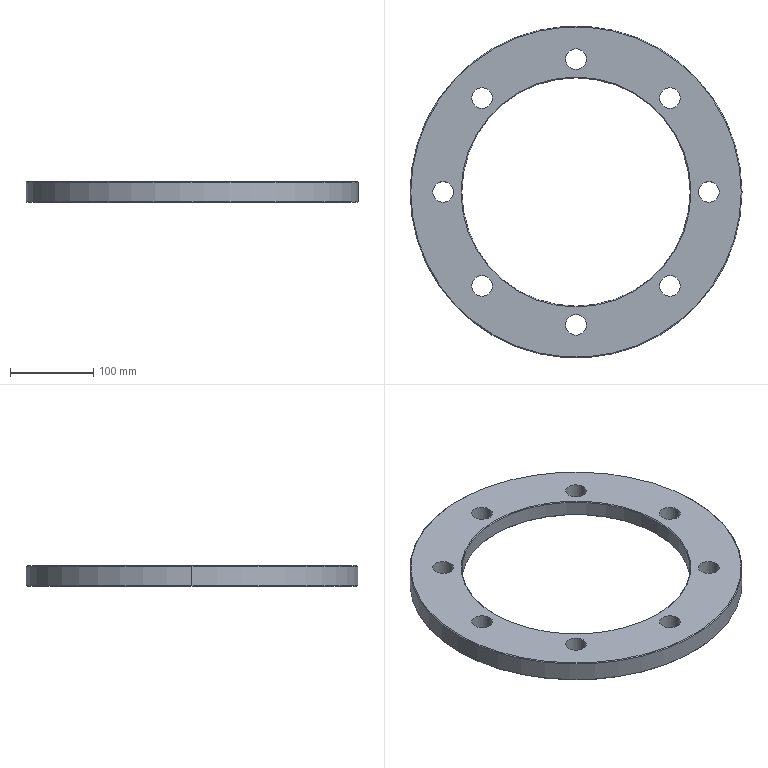Part | SolidWorks | features Chamfer 2, Extrusion 1, Fillet 1, ICE 1 | 1 solid | 37 faces | box 400 x 400 x 25 mm | volume 1378515 mm3 | cylinder 22 | cone 10 | plane 3 | torus 2 | commonest cylinder face diameters 25 x16 275 x2 355 x2 400 x2
STEP:
#1=CARTESIAN_POINT('',(177.5,0.,1.));
#2=VERTEX_POINT('',#1);
#3=CARTESIAN_POINT('',(-177.5,0.,1.));
#4=VERTEX_POINT('',#3);
#5=CARTESIAN_POINT('',(0.,0.,1.));
#6=DIRECTION('',(0.,0.,-1.));
#7=DIRECTION('',(1.,0.,0.));
#8=AXIS2_PLACEMENT_3D('',#5,#6,#7);
#9=CIRCLE('',#8,177.5);
#10=EDGE_CURVE('',#2,#4,#9,.T.);
#11=ORIENTED_EDGE('',*,*,#10,.F.);
#12=CARTESIAN_POINT('',(178.5,0.,0.));
#13=VERTEX_POINT('',#12);
#14=CARTESIAN_POINT('',(177.5,0.,1.));
#15=DIRECTION('',(0.7071,0.,-0.7071));
#16=VECTOR('',#15,1000.);
#17=LINE('',#14,#16);
#18=EDGE_CURVE('',#2,#13,#17,.T.);
#19=ORIENTED_EDGE('',*,*,#18,.T.);
#20=CARTESIAN_POINT('',(-178.5,0.,0.));
#21=VERTEX_POINT('',#20);
#22=CARTESIAN_POINT('',(0.,0.,0.));
#23=DIRECTION('',(0.,0.,1.));
#24=DIRECTION('',(1.,0.,0.));
#25=AXIS2_PLACEMENT_3D('',#22,#23,#24);
#26=CIRCLE('',#25,178.5);
#27=EDGE_CURVE('',#21,#13,#26,.T.);
#28=ORIENTED_EDGE('',*,*,#27,.F.);
#29=CARTESIAN_POINT('',(-177.5,0.,1.));
#30=DIRECTION('',(-0.7071,0.,-0.7071));
#31=VECTOR('',#30,1000.);
#32=LINE('',#29,#31);
#33=EDGE_CURVE('',#4,#21,#32,.T.);
#34=ORIENTED_EDGE('',*,*,#33,.F.);
#35=EDGE_LOOP('',(#11,#19,#28,#34));
#36=FACE_OUTER_BOUND('',#35,.T.);
#37=CARTESIAN_POINT('',(0.,0.,1.));
#38=DIRECTION('',(0.,0.,-1.));
#39=DIRECTION('',(-1.,0.,0.));
#40=AXIS2_PLACEMENT_3D('',#37,#38,#39);
#41=CONICAL_SURFACE('',#40,177.5,0.7854);
#42=ADVANCED_FACE('',(#36),#41,.F.);
#43=CARTESIAN_POINT('',(137.5,0.,6.));
#44=VERTEX_POINT('',#43);
#45=CARTESIAN_POINT('',(-137.5,0.,6.));
#46=VERTEX_POINT('',#45);
#47=CARTESIAN_POINT('',(0.,0.,6.));
#48=DIRECTION('',(0.,0.,-1.));
#49=DIRECTION('',(-1.,0.,0.));
#50=AXIS2_PLACEMENT_3D('',#47,#48,#49);
#51=CIRCLE('',#50,137.5);
#52=EDGE_CURVE('',#44,#46,#51,.T.);
#53=ORIENTED_EDGE('',*,*,#52,.F.);
#54=CARTESIAN_POINT('',(138.5,0.,5.));
#55=VERTEX_POINT('',#54);
#56=CARTESIAN_POINT('',(137.5,0.,6.));
#57=DIRECTION('',(0.7071,0.,-0.7071));
#58=VECTOR('',#57,1000.);
#59=LINE('',#56,#58);
#60=EDGE_CURVE('',#44,#55,#59,.T.);
#61=ORIENTED_EDGE('',*,*,#60,.T.);
#62=CARTESIAN_POINT('',(-138.5,0.,5.));
#63=VERTEX_POINT('',#62);
#64=CARTESIAN_POINT('',(0.,0.,5.));
#65=DIRECTION('',(0.,0.,1.));
#66=DIRECTION('',(-1.,0.,0.));
#67=AXIS2_PLACEMENT_3D('',#64,#65,#66);
#68=CIRCLE('',#67,138.5);
#69=EDGE_CURVE('',#63,#55,#68,.T.);
#70=ORIENTED_EDGE('',*,*,#69,.F.);
#71=CARTESIAN_POINT('',(-137.5,0.,6.));
#72=DIRECTION('',(-0.7071,0.,-0.7071));
#73=VECTOR('',#72,1000.);
#74=LINE('',#71,#73);
#75=EDGE_CURVE('',#46,#63,#74,.T.);
#76=ORIENTED_EDGE('',*,*,#75,.F.);
#77=EDGE_LOOP('',(#53,#61,#70,#76));
#78=FACE_OUTER_BOUND('',#77,.T.);
#79=CARTESIAN_POINT('',(0.,0.,6.));
#80=DIRECTION('',(0.,0.,-1.));
#81=DIRECTION('',(-1.,0.,0.));
#82=AXIS2_PLACEMENT_3D('',#79,#80,#81);
#83=CONICAL_SURFACE('',#82,137.5,0.7854);
#84=ADVANCED_FACE('',(#78),#83,.F.);
#85=CARTESIAN_POINT('',(175.5,0.,5.));
#86=VERTEX_POINT('',#85);
#87=CARTESIAN_POINT('',(-175.5,0.,5.));
#88=VERTEX_POINT('',#87);
#89=CARTESIAN_POINT('',(0.,0.,5.));
#90=DIRECTION('',(0.,0.,-1.));
#91=DIRECTION('',(-1.,0.,0.));
#92=AXIS2_PLACEMENT_3D('',#89,#90,#91);
#93=CIRCLE('',#92,175.5);
#94=EDGE_CURVE('',#86,#88,#93,.T.);
#95=ORIENTED_EDGE('',*,*,#94,.F.);
#96=CARTESIAN_POINT('',(177.5,0.,3.));
#97=VERTEX_POINT('',#96);
#98=CARTESIAN_POINT('',(175.5,0.,3.));
#99=DIRECTION('',(0.,1.,0.));
#100=DIRECTION('',(-1.,0.,0.));
#101=AXIS2_PLACEMENT_3D('',#98,#99,#100);
#102=CIRCLE('',#101,2.);
#103=EDGE_CURVE('',#86,#97,#102,.T.);
#104=ORIENTED_EDGE('',*,*,#103,.T.);
#105=CARTESIAN_POINT('',(-177.5,0.,3.));
#106=VERTEX_POINT('',#105);
#107=CARTESIAN_POINT('',(0.,0.,3.));
#108=DIRECTION('',(0.,0.,1.));
#109=DIRECTION('',(-1.,0.,0.));
#110=AXIS2_PLACEMENT_3D('',#107,#108,#109);
#111=CIRCLE('',#110,177.5);
#112=EDGE_CURVE('',#106,#97,#111,.T.);
#113=ORIENTED_EDGE('',*,*,#112,.F.);
#114=CARTESIAN_POINT('',(-175.5,0.,3.));
#115=DIRECTION('',(0.,-1.,0.));
#116=DIRECTION('',(1.,0.,0.));
#117=AXIS2_PLACEMENT_3D('',#114,#115,#116);
#118=CIRCLE('',#117,2.);
#119=EDGE_CURVE('',#88,#106,#118,.T.);
#120=ORIENTED_EDGE('',*,*,#119,.F.);
#121=EDGE_LOOP('',(#95,#104,#113,#120));
#122=FACE_OUTER_BOUND('',#121,.T.);
#123=CARTESIAN_POINT('',(0.,0.,3.));
#124=DIRECTION('',(0.,0.,-1.));
#125=DIRECTION('',(-1.,0.,0.));
#126=AXIS2_PLACEMENT_3D('',#123,#124,#125);
#127=TOROIDAL_SURFACE('',#126,175.5,2.);
#128=ADVANCED_FACE('',(#122),#127,.F.);
#129=ORIENTED_EDGE('',*,*,#112,.T.);
#130=CARTESIAN_POINT('',(177.5,0.,5.));
#131=DIRECTION('',(0.,0.,-1.));
#132=VECTOR('',#131,1000.);
#133=LINE('',#130,#132);
#134=EDGE_CURVE('',#97,#2,#133,.T.);
#135=ORIENTED_EDGE('',*,*,#134,.T.);
#136=ORIENTED_EDGE('',*,*,#10,.T.);
#137=CARTESIAN_POINT('',(-177.5,0.,5.));
#138=DIRECTION('',(0.,0.,-1.));
#139=VECTOR('',#138,1000.);
#140=LINE('',#137,#139);
#141=EDGE_CURVE('',#106,#4,#140,.T.);
#142=ORIENTED_EDGE('',*,*,#141,.F.);
#143=EDGE_LOOP('',(#129,#135,#136,#142));
#144=FACE_OUTER_BOUND('',#143,.T.);
#145=CARTESIAN_POINT('',(0.,0.,5.));
#146=DIRECTION('',(0.,0.,-1.));
#147=DIRECTION('',(-1.,0.,0.));
#148=AXIS2_PLACEMENT_3D('',#145,#146,#147);
#149=CYLINDRICAL_SURFACE('',#148,177.5);
#150=ADVANCED_FACE('',(#144),#149,.F.);
#151=CARTESIAN_POINT('',(199.,0.,25.));
#152=VERTEX_POINT('',#151);
#153=CARTESIAN_POINT('',(-199.,0.,25.));
#154=VERTEX_POINT('',#153);
#155=CARTESIAN_POINT('',(0.,0.,25.));
#156=DIRECTION('',(0.,0.,1.));
#157=DIRECTION('',(1.,0.,0.));
#158=AXIS2_PLACEMENT_3D('',#155,#156,#157);
#159=CIRCLE('',#158,199.);
#160=EDGE_CURVE('',#152,#154,#159,.T.);
#161=ORIENTED_EDGE('',*,*,#160,.F.);
#162=CARTESIAN_POINT('',(200.,0.,24.));
#163=VERTEX_POINT('',#162);
#164=CARTESIAN_POINT('',(199.,0.,25.));
#165=DIRECTION('',(0.7071,0.,-0.7071));
#166=VECTOR('',#165,1000.);
#167=LINE('',#164,#166);
#168=EDGE_CURVE('',#152,#163,#167,.T.);
#169=ORIENTED_EDGE('',*,*,#168,.T.);
#170=CARTESIAN_POINT('',(-200.,0.,24.));
#171=VERTEX_POINT('',#170);
#172=CARTESIAN_POINT('',(0.,0.,24.));
#173=DIRECTION('',(0.,0.,-1.));
#174=DIRECTION('',(1.,0.,0.));
#175=AXIS2_PLACEMENT_3D('',#172,#173,#174);
#176=CIRCLE('',#175,200.);
#177=EDGE_CURVE('',#171,#163,#176,.T.);
#178=ORIENTED_EDGE('',*,*,#177,.F.);
#179=CARTESIAN_POINT('',(-199.,0.,25.));
#180=DIRECTION('',(-0.7071,0.,-0.7071));
#181=VECTOR('',#180,1000.);
#182=LINE('',#179,#181);
#183=EDGE_CURVE('',#154,#171,#182,.T.);
#184=ORIENTED_EDGE('',*,*,#183,.F.);
#185=EDGE_LOOP('',(#161,#169,#178,#184));
#186=FACE_OUTER_BOUND('',#185,.T.);
#187=CARTESIAN_POINT('',(0.,0.,25.));
#188=DIRECTION('',(0.,0.,-1.));
#189=DIRECTION('',(-1.,0.,0.));
#190=AXIS2_PLACEMENT_3D('',#187,#188,#189);
#191=CONICAL_SURFACE('',#190,199.,0.7854);
#192=ADVANCED_FACE('',(#186),#191,.T.);
#193=CARTESIAN_POINT('',(-199.,0.,0.));
#194=VERTEX_POINT('',#193);
#195=CARTESIAN_POINT('',(199.,0.,0.));
#196=VERTEX_POINT('',#195);
#197=CARTESIAN_POINT('',(0.,0.,0.));
#198=DIRECTION('',(0.,0.,-1.));
#199=DIRECTION('',(1.,0.,0.));
#200=AXIS2_PLACEMENT_3D('',#197,#198,#199);
#201=CIRCLE('',#200,199.);
#202=EDGE_CURVE('',#194,#196,#201,.T.);
#203=ORIENTED_EDGE('',*,*,#202,.F.);
#204=CARTESIAN_POINT('',(-200.,0.,1.));
#205=VERTEX_POINT('',#204);
#206=CARTESIAN_POINT('',(-200.,0.,1.));
#207=DIRECTION('',(-0.7071,0.,0.7071));
#208=VECTOR('',#207,1000.);
#209=LINE('',#206,#208);
#210=EDGE_CURVE('',#194,#205,#209,.T.);
#211=ORIENTED_EDGE('',*,*,#210,.T.);
#212=CARTESIAN_POINT('',(200.,0.,1.));
#213=VERTEX_POINT('',#212);
#214=CARTESIAN_POINT('',(0.,0.,1.));
#215=DIRECTION('',(0.,0.,1.));
#216=DIRECTION('',(1.,0.,0.));
#217=AXIS2_PLACEMENT_3D('',#214,#215,#216);
#218=CIRCLE('',#217,200.);
#219=EDGE_CURVE('',#213,#205,#218,.T.);
#220=ORIENTED_EDGE('',*,*,#219,.F.);
#221=CARTESIAN_POINT('',(200.,0.,1.));
#222=DIRECTION('',(0.7071,0.,0.7071));
#223=VECTOR('',#222,1000.);
#224=LINE('',#221,#223);
#225=EDGE_CURVE('',#196,#213,#224,.T.);
#226=ORIENTED_EDGE('',*,*,#225,.F.);
#227=EDGE_LOOP('',(#203,#211,#220,#226));
#228=FACE_OUTER_BOUND('',#227,.T.);
#229=CARTESIAN_POINT('',(0.,0.,1.));
#230=DIRECTION('',(0.,0.,1.));
#231=DIRECTION('',(1.,0.,0.));
#232=AXIS2_PLACEMENT_3D('',#229,#230,#231);
#233=CONICAL_SURFACE('',#232,200.,0.7854);
#234=ADVANCED_FACE('',(#228),#233,.T.);
#235=CARTESIAN_POINT('',(-137.5,0.,24.));
#236=VERTEX_POINT('',#235);
#237=CARTESIAN_POINT('',(137.5,0.,24.));
#238=VERTEX_POINT('',#237);
#239=CARTESIAN_POINT('',(0.,0.,24.));
#240=DIRECTION('',(0.,0.,1.));
#241=DIRECTION('',(1.,0.,0.));
#242=AXIS2_PLACEMENT_3D('',#239,#240,#241);
#243=CIRCLE('',#242,137.5);
#244=EDGE_CURVE('',#236,#238,#243,.T.);
#245=ORIENTED_EDGE('',*,*,#244,.F.);
#246=CARTESIAN_POINT('',(-138.5,0.,25.));
#247=VERTEX_POINT('',#246);
#248=CARTESIAN_POINT('',(-137.5,0.,24.));
#249=DIRECTION('',(-0.7071,0.,0.7071));
#250=VECTOR('',#249,1000.);
#251=LINE('',#248,#250);
#252=EDGE_CURVE('',#236,#247,#251,.T.);
#253=ORIENTED_EDGE('',*,*,#252,.T.);
#254=CARTESIAN_POINT('',(138.5,0.,25.));
#255=VERTEX_POINT('',#254);
#256=CARTESIAN_POINT('',(0.,0.,25.));
#257=DIRECTION('',(0.,0.,-1.));
#258=DIRECTION('',(1.,0.,0.));
#259=AXIS2_PLACEMENT_3D('',#256,#257,#258);
#260=CIRCLE('',#259,138.5);
#261=EDGE_CURVE('',#255,#247,#260,.T.);
#262=ORIENTED_EDGE('',*,*,#261,.F.);
#263=CARTESIAN_POINT('',(137.5,0.,24.));
#264=DIRECTION('',(0.7071,0.,0.7071));
#265=VECTOR('',#264,1000.);
#266=LINE('',#263,#265);
#267=EDGE_CURVE('',#238,#255,#266,.T.);
#268=ORIENTED_EDGE('',*,*,#267,.F.);
#269=EDGE_LOOP('',(#245,#253,#262,#268));
#270=FACE_OUTER_BOUND('',#269,.T.);
#271=CARTESIAN_POINT('',(0.,0.,24.));
#272=DIRECTION('',(0.,0.,1.));
#273=DIRECTION('',(1.,0.,0.));
#274=AXIS2_PLACEMENT_3D('',#271,#272,#273);
#275=CONICAL_SURFACE('',#274,137.5,0.7854);
#276=ADVANCED_FACE('',(#270),#275,.F.);
#277=ORIENTED_EDGE('',*,*,#177,.T.);
#278=CARTESIAN_POINT('',(200.,0.,25.));
#279=DIRECTION('',(0.,0.,-1.));
#280=VECTOR('',#279,1000.);
#281=LINE('',#278,#280);
#282=EDGE_CURVE('',#163,#213,#281,.T.);
#283=ORIENTED_EDGE('',*,*,#282,.T.);
#284=ORIENTED_EDGE('',*,*,#219,.T.);
#285=CARTESIAN_POINT('',(-200.,0.,25.));
#286=DIRECTION('',(0.,0.,-1.));
#287=VECTOR('',#286,1000.);
#288=LINE('',#285,#287);
#289=EDGE_CURVE('',#171,#205,#288,.T.);
#290=ORIENTED_EDGE('',*,*,#289,.F.);
#291=EDGE_LOOP('',(#277,#283,#284,#290));
#292=FACE_OUTER_BOUND('',#291,.T.);
#293=CARTESIAN_POINT('',(0.,0.,25.));
#294=DIRECTION('',(0.,0.,-1.));
#295=DIRECTION('',(-1.,0.,0.));
#296=AXIS2_PLACEMENT_3D('',#293,#294,#295);
#297=CYLINDRICAL_SURFACE('',#296,200.);
#298=ADVANCED_FACE('',(#292),#297,.T.);
#299=CARTESIAN_POINT('',(-125.637,113.137,25.));
#300=VERTEX_POINT('',#299);
#301=CARTESIAN_POINT('',(-100.637,113.137,25.));
#302=VERTEX_POINT('',#301);
#303=CARTESIAN_POINT('',(-113.137,113.137,25.));
#304=DIRECTION('',(0.,0.,1.));
#305=DIRECTION('',(1.,0.,0.));
#306=AXIS2_PLACEMENT_3D('',#303,#304,#305);
#307=CIRCLE('',#306,12.5);
#308=EDGE_CURVE('',#300,#302,#307,.T.);
#309=ORIENTED_EDGE('',*,*,#308,.T.);
#310=CARTESIAN_POINT('',(-100.637,113.137,5.));
#311=VERTEX_POINT('',#310);
#312=CARTESIAN_POINT('',(-100.637,113.137,25.));
#313=DIRECTION('',(0.,0.,-1.));
#314=VECTOR('',#313,1000.);
#315=LINE('',#312,#314);
#316=EDGE_CURVE('',#302,#311,#315,.T.);
#317=ORIENTED_EDGE('',*,*,#316,.T.);
#318=CARTESIAN_POINT('',(-125.637,113.137,5.));
#319=VERTEX_POINT('',#318);
#320=CARTESIAN_POINT('',(-113.137,113.137,5.));
#321=DIRECTION('',(0.,0.,-1.));
#322=DIRECTION('',(-1.,0.,0.));
#323=AXIS2_PLACEMENT_3D('',#320,#321,#322);
#324=CIRCLE('',#323,12.5);
#325=EDGE_CURVE('',#311,#319,#324,.T.);
#326=ORIENTED_EDGE('',*,*,#325,.T.);
#327=CARTESIAN_POINT('',(-125.637,113.137,25.));
#328=DIRECTION('',(0.,0.,-1.));
#329=VECTOR('',#328,1000.);
#330=LINE('',#327,#329);
#331=EDGE_CURVE('',#300,#319,#330,.T.);
#332=ORIENTED_EDGE('',*,*,#331,.F.);
#333=EDGE_LOOP('',(#309,#317,#326,#332));
#334=FACE_OUTER_BOUND('',#333,.T.);
#335=CARTESIAN_POINT('',(-113.137,113.137,25.));
#336=DIRECTION('',(0.,0.,-1.));
#337=DIRECTION('',(-1.,0.,0.));
#338=AXIS2_PLACEMENT_3D('',#335,#336,#337);
#339=CYLINDRICAL_SURFACE('',#338,12.5);
#340=ADVANCED_FACE('',(#334),#339,.F.);
#341=CARTESIAN_POINT('',(-172.5,0.,25.));
#342=VERTEX_POINT('',#341);
#343=CARTESIAN_POINT('',(-147.5,0.,25.));
#344=VERTEX_POINT('',#343);
#345=CARTESIAN_POINT('',(-160.,0.,25.));
#346=DIRECTION('',(0.,0.,1.));
#347=DIRECTION('',(1.,0.,0.));
#348=AXIS2_PLACEMENT_3D('',#345,#346,#347);
#349=CIRCLE('',#348,12.5);
#350=EDGE_CURVE('',#342,#344,#349,.T.);
#351=ORIENTED_EDGE('',*,*,#350,.T.);
#352=CARTESIAN_POINT('',(-147.5,0.,5.));
#353=VERTEX_POINT('',#352);
#354=CARTESIAN_POINT('',(-147.5,0.,25.));
#355=DIRECTION('',(0.,0.,-1.));
#356=VECTOR('',#355,1000.);
#357=LINE('',#354,#356);
#358=EDGE_CURVE('',#344,#353,#357,.T.);
#359=ORIENTED_EDGE('',*,*,#358,.T.);
#360=CARTESIAN_POINT('',(-172.5,0.,5.));
#361=VERTEX_POINT('',#360);
#362=CARTESIAN_POINT('',(-160.,0.,5.));
#363=DIRECTION('',(0.,0.,-1.));
#364=DIRECTION('',(-1.,0.,0.));
#365=AXIS2_PLACEMENT_3D('',#362,#363,#364);
#366=CIRCLE('',#365,12.5);
#367=EDGE_CURVE('',#353,#361,#366,.T.);
#368=ORIENTED_EDGE('',*,*,#367,.T.);
#369=CARTESIAN_POINT('',(-172.5,0.,25.));
#370=DIRECTION('',(0.,0.,-1.));
#371=VECTOR('',#370,1000.);
#372=LINE('',#369,#371);
#373=EDGE_CURVE('',#342,#361,#372,.T.);
#374=ORIENTED_EDGE('',*,*,#373,.F.);
#375=EDGE_LOOP('',(#351,#359,#368,#374));
#376=FACE_OUTER_BOUND('',#375,.T.);
#377=CARTESIAN_POINT('',(-160.,0.,25.));
#378=DIRECTION('',(0.,0.,-1.));
#379=DIRECTION('',(-1.,0.,0.));
#380=AXIS2_PLACEMENT_3D('',#377,#378,#379);
#381=CYLINDRICAL_SURFACE('',#380,12.5);
#382=ADVANCED_FACE('',(#376),#381,.F.);
#383=CARTESIAN_POINT('',(-125.637,-113.137,25.));
#384=VERTEX_POINT('',#383);
#385=CARTESIAN_POINT('',(-100.637,-113.137,25.));
#386=VERTEX_POINT('',#385);
#387=CARTESIAN_POINT('',(-113.137,-113.137,25.));
#388=DIRECTION('',(0.,0.,1.));
#389=DIRECTION('',(1.,0.,0.));
#390=AXIS2_PLACEMENT_3D('',#387,#388,#389);
#391=CIRCLE('',#390,12.5);
#392=EDGE_CURVE('',#384,#386,#391,.T.);
#393=ORIENTED_EDGE('',*,*,#392,.T.);
#394=CARTESIAN_POINT('',(-100.637,-113.137,5.));
#395=VERTEX_POINT('',#394);
#396=CARTESIAN_POINT('',(-100.637,-113.137,25.));
#397=DIRECTION('',(0.,0.,-1.));
#398=VECTOR('',#397,1000.);
#399=LINE('',#396,#398);
#400=EDGE_CURVE('',#386,#395,#399,.T.);
#401=ORIENTED_EDGE('',*,*,#400,.T.);
#402=CARTESIAN_POINT('',(-125.637,-113.137,5.));
#403=VERTEX_POINT('',#402);
#404=CARTESIAN_POINT('',(-113.137,-113.137,5.));
#405=DIRECTION('',(0.,0.,-1.));
#406=DIRECTION('',(-1.,0.,0.));
#407=AXIS2_PLACEMENT_3D('',#404,#405,#406);
#408=CIRCLE('',#407,12.5);
#409=EDGE_CURVE('',#395,#403,#408,.T.);
#410=ORIENTED_EDGE('',*,*,#409,.T.);
#411=CARTESIAN_POINT('',(-125.637,-113.137,25.));
#412=DIRECTION('',(0.,0.,-1.));
#413=VECTOR('',#412,1000.);
#414=LINE('',#411,#413);
#415=EDGE_CURVE('',#384,#403,#414,.T.);
#416=ORIENTED_EDGE('',*,*,#415,.F.);
#417=EDGE_LOOP('',(#393,#401,#410,#416));
#418=FACE_OUTER_BOUND('',#417,.T.);
#419=CARTESIAN_POINT('',(-113.137,-113.137,25.));
#420=DIRECTION('',(0.,0.,-1.));
#421=DIRECTION('',(-1.,0.,0.));
#422=AXIS2_PLACEMENT_3D('',#419,#420,#421);
#423=CYLINDRICAL_SURFACE('',#422,12.5);
#424=ADVANCED_FACE('',(#418),#423,.F.);
#425=CARTESIAN_POINT('',(-12.5,-160.,25.));
#426=VERTEX_POINT('',#425);
#427=CARTESIAN_POINT('',(12.5,-160.,25.));
#428=VERTEX_POINT('',#427);
#429=CARTESIAN_POINT('',(0.,-160.,25.));
#430=DIRECTION('',(0.,0.,1.));
#431=DIRECTION('',(1.,0.,0.));
#432=AXIS2_PLACEMENT_3D('',#429,#430,#431);
#433=CIRCLE('',#432,12.5);
#434=EDGE_CURVE('',#426,#428,#433,.T.);
#435=ORIENTED_EDGE('',*,*,#434,.T.);
#436=CARTESIAN_POINT('',(12.5,-160.,5.));
#437=VERTEX_POINT('',#436);
#438=CARTESIAN_POINT('',(12.5,-160.,25.));
#439=DIRECTION('',(0.,0.,-1.));
#440=VECTOR('',#439,1000.);
#441=LINE('',#438,#440);
#442=EDGE_CURVE('',#428,#437,#441,.T.);
#443=ORIENTED_EDGE('',*,*,#442,.T.);
#444=CARTESIAN_POINT('',(-12.5,-160.,5.));
#445=VERTEX_POINT('',#444);
#446=CARTESIAN_POINT('',(0.,-160.,5.));
#447=DIRECTION('',(0.,0.,-1.));
#448=DIRECTION('',(-1.,0.,0.));
#449=AXIS2_PLACEMENT_3D('',#446,#447,#448);
#450=CIRCLE('',#449,12.5);
#451=EDGE_CURVE('',#437,#445,#450,.T.);
#452=ORIENTED_EDGE('',*,*,#451,.T.);
#453=CARTESIAN_POINT('',(-12.5,-160.,25.));
#454=DIRECTION('',(0.,0.,-1.));
#455=VECTOR('',#454,1000.);
#456=LINE('',#453,#455);
#457=EDGE_CURVE('',#426,#445,#456,.T.);
#458=ORIENTED_EDGE('',*,*,#457,.F.);
#459=EDGE_LOOP('',(#435,#443,#452,#458));
#460=FACE_OUTER_BOUND('',#459,.T.);
#461=CARTESIAN_POINT('',(0.,-160.,25.));
#462=DIRECTION('',(0.,0.,-1.));
#463=DIRECTION('',(-1.,0.,0.));
#464=AXIS2_PLACEMENT_3D('',#461,#462,#463);
#465=CYLINDRICAL_SURFACE('',#464,12.5);
#466=ADVANCED_FACE('',(#460),#465,.F.);
#467=CARTESIAN_POINT('',(100.637,-113.137,25.));
#468=VERTEX_POINT('',#467);
#469=CARTESIAN_POINT('',(125.637,-113.137,25.));
#470=VERTEX_POINT('',#469);
#471=CARTESIAN_POINT('',(113.137,-113.137,25.));
#472=DIRECTION('',(0.,0.,1.));
#473=DIRECTION('',(1.,0.,0.));
#474=AXIS2_PLACEMENT_3D('',#471,#472,#473);
#475=CIRCLE('',#474,12.5);
#476=EDGE_CURVE('',#468,#470,#475,.T.);
#477=ORIENTED_EDGE('',*,*,#476,.T.);
#478=CARTESIAN_POINT('',(125.637,-113.137,5.));
#479=VERTEX_POINT('',#478);
#480=CARTESIAN_POINT('',(125.637,-113.137,25.));
#481=DIRECTION('',(0.,0.,-1.));
#482=VECTOR('',#481,1000.);
#483=LINE('',#480,#482);
#484=EDGE_CURVE('',#470,#479,#483,.T.);
#485=ORIENTED_EDGE('',*,*,#484,.T.);
#486=CARTESIAN_POINT('',(100.637,-113.137,5.));
#487=VERTEX_POINT('',#486);
#488=CARTESIAN_POINT('',(113.137,-113.137,5.));
#489=DIRECTION('',(0.,0.,-1.));
#490=DIRECTION('',(-1.,0.,0.));
#491=AXIS2_PLACEMENT_3D('',#488,#489,#490);
#492=CIRCLE('',#491,12.5);
#493=EDGE_CURVE('',#479,#487,#492,.T.);
#494=ORIENTED_EDGE('',*,*,#493,.T.);
#495=CARTESIAN_POINT('',(100.637,-113.137,25.));
#496=DIRECTION('',(0.,0.,-1.));
#497=VECTOR('',#496,1000.);
#498=LINE('',#495,#497);
#499=EDGE_CURVE('',#468,#487,#498,.T.);
#500=ORIENTED_EDGE('',*,*,#499,.F.);
#501=EDGE_LOOP('',(#477,#485,#494,#500));
#502=FACE_OUTER_BOUND('',#501,.T.);
#503=CARTESIAN_POINT('',(113.137,-113.137,25.));
#504=DIRECTION('',(0.,0.,-1.));
#505=DIRECTION('',(-1.,0.,0.));
#506=AXIS2_PLACEMENT_3D('',#503,#504,#505);
#507=CYLINDRICAL_SURFACE('',#506,12.5);
#508=ADVANCED_FACE('',(#502),#507,.F.);
#509=CARTESIAN_POINT('',(147.5,0.,25.));
#510=VERTEX_POINT('',#509);
#511=CARTESIAN_POINT('',(172.5,0.,25.));
#512=VERTEX_POINT('',#511);
#513=CARTESIAN_POINT('',(160.,0.,25.));
#514=DIRECTION('',(0.,0.,1.));
#515=DIRECTION('',(1.,0.,0.));
#516=AXIS2_PLACEMENT_3D('',#513,#514,#515);
#517=CIRCLE('',#516,12.5);
#518=EDGE_CURVE('',#510,#512,#517,.T.);
#519=ORIENTED_EDGE('',*,*,#518,.T.);
#520=CARTESIAN_POINT('',(172.5,0.,5.));
#521=VERTEX_POINT('',#520);
#522=CARTESIAN_POINT('',(172.5,0.,25.));
#523=DIRECTION('',(0.,0.,-1.));
#524=VECTOR('',#523,1000.);
#525=LINE('',#522,#524);
#526=EDGE_CURVE('',#512,#521,#525,.T.);
#527=ORIENTED_EDGE('',*,*,#526,.T.);
#528=CARTESIAN_POINT('',(147.5,0.,5.));
#529=VERTEX_POINT('',#528);
#530=CARTESIAN_POINT('',(160.,0.,5.));
#531=DIRECTION('',(0.,0.,-1.));
#532=DIRECTION('',(-1.,0.,0.));
#533=AXIS2_PLACEMENT_3D('',#530,#531,#532);
#534=CIRCLE('',#533,12.5);
#535=EDGE_CURVE('',#521,#529,#534,.T.);
#536=ORIENTED_EDGE('',*,*,#535,.T.);
#537=CARTESIAN_POINT('',(147.5,0.,25.));
#538=DIRECTION('',(0.,0.,-1.));
#539=VECTOR('',#538,1000.);
#540=LINE('',#537,#539);
#541=EDGE_CURVE('',#510,#529,#540,.T.);
#542=ORIENTED_EDGE('',*,*,#541,.F.);
#543=EDGE_LOOP('',(#519,#527,#536,#542));
#544=FACE_OUTER_BOUND('',#543,.T.);
#545=CARTESIAN_POINT('',(160.,0.,25.));
#546=DIRECTION('',(0.,0.,-1.));
#547=DIRECTION('',(-1.,0.,0.));
#548=AXIS2_PLACEMENT_3D('',#545,#546,#547);
#549=CYLINDRICAL_SURFACE('',#548,12.5);
#550=ADVANCED_FACE('',(#544),#549,.F.);
#551=CARTESIAN_POINT('',(100.637,113.137,25.));
#552=VERTEX_POINT('',#551);
#553=CARTESIAN_POINT('',(125.637,113.137,25.));
#554=VERTEX_POINT('',#553);
#555=CARTESIAN_POINT('',(113.137,113.137,25.));
#556=DIRECTION('',(0.,0.,1.));
#557=DIRECTION('',(1.,0.,0.));
#558=AXIS2_PLACEMENT_3D('',#555,#556,#557);
#559=CIRCLE('',#558,12.5);
#560=EDGE_CURVE('',#552,#554,#559,.T.);
#561=ORIENTED_EDGE('',*,*,#560,.T.);
#562=CARTESIAN_POINT('',(125.637,113.137,5.));
#563=VERTEX_POINT('',#562);
#564=CARTESIAN_POINT('',(125.637,113.137,25.));
#565=DIRECTION('',(0.,0.,-1.));
#566=VECTOR('',#565,1000.);
#567=LINE('',#564,#566);
#568=EDGE_CURVE('',#554,#563,#567,.T.);
#569=ORIENTED_EDGE('',*,*,#568,.T.);
#570=CARTESIAN_POINT('',(100.637,113.137,5.));
#571=VERTEX_POINT('',#570);
#572=CARTESIAN_POINT('',(113.137,113.137,5.));
#573=DIRECTION('',(0.,0.,-1.));
#574=DIRECTION('',(-1.,0.,0.));
#575=AXIS2_PLACEMENT_3D('',#572,#573,#574);
#576=CIRCLE('',#575,12.5);
#577=EDGE_CURVE('',#563,#571,#576,.T.);
#578=ORIENTED_EDGE('',*,*,#577,.T.);
#579=CARTESIAN_POINT('',(100.637,113.137,25.));
#580=DIRECTION('',(0.,0.,-1.));
#581=VECTOR('',#580,1000.);
#582=LINE('',#579,#581);
#583=EDGE_CURVE('',#552,#571,#582,.T.);
#584=ORIENTED_EDGE('',*,*,#583,.F.);
#585=EDGE_LOOP('',(#561,#569,#578,#584));
#586=FACE_OUTER_BOUND('',#585,.T.);
#587=CARTESIAN_POINT('',(113.137,113.137,25.));
#588=DIRECTION('',(0.,0.,-1.));
#589=DIRECTION('',(-1.,0.,0.));
#590=AXIS2_PLACEMENT_3D('',#587,#588,#589);
#591=CYLINDRICAL_SURFACE('',#590,12.5);
#592=ADVANCED_FACE('',(#586),#591,.F.);
#593=CARTESIAN_POINT('',(-12.5,160.,25.));
#594=VERTEX_POINT('',#593);
#595=CARTESIAN_POINT('',(12.5,160.,25.));
#596=VERTEX_POINT('',#595);
#597=CARTESIAN_POINT('',(0.,160.,25.));
#598=DIRECTION('',(0.,0.,1.));
#599=DIRECTION('',(1.,0.,0.));
#600=AXIS2_PLACEMENT_3D('',#597,#598,#599);
#601=CIRCLE('',#600,12.5);
#602=EDGE_CURVE('',#594,#596,#601,.T.);
#603=ORIENTED_EDGE('',*,*,#602,.T.);
#604=CARTESIAN_POINT('',(12.5,160.,5.));
#605=VERTEX_POINT('',#604);
#606=CARTESIAN_POINT('',(12.5,160.,25.));
#607=DIRECTION('',(0.,0.,-1.));
#608=VECTOR('',#607,1000.);
#609=LINE('',#606,#608);
#610=EDGE_CURVE('',#596,#605,#609,.T.);
#611=ORIENTED_EDGE('',*,*,#610,.T.);
#612=CARTESIAN_POINT('',(-12.5,160.,5.));
#613=VERTEX_POINT('',#612);
#614=CARTESIAN_POINT('',(0.,160.,5.));
#615=DIRECTION('',(0.,0.,-1.));
#616=DIRECTION('',(-1.,0.,0.));
#617=AXIS2_PLACEMENT_3D('',#614,#615,#616);
#618=CIRCLE('',#617,12.5);
#619=EDGE_CURVE('',#605,#613,#618,.T.);
#620=ORIENTED_EDGE('',*,*,#619,.T.);
#621=CARTESIAN_POINT('',(-12.5,160.,25.));
#622=DIRECTION('',(0.,0.,-1.));
#623=VECTOR('',#622,1000.);
#624=LINE('',#621,#623);
#625=EDGE_CURVE('',#594,#613,#624,.T.);
#626=ORIENTED_EDGE('',*,*,#625,.F.);
#627=EDGE_LOOP('',(#603,#611,#620,#626));
#628=FACE_OUTER_BOUND('',#627,.T.);
#629=CARTESIAN_POINT('',(0.,160.,25.));
#630=DIRECTION('',(0.,0.,-1.));
#631=DIRECTION('',(-1.,0.,0.));
#632=AXIS2_PLACEMENT_3D('',#629,#630,#631);
#633=CYLINDRICAL_SURFACE('',#632,12.5);
#634=ADVANCED_FACE('',(#628),#633,.F.);
#635=ORIENTED_EDGE('',*,*,#244,.T.);
#636=CARTESIAN_POINT('',(137.5,0.,25.));
#637=DIRECTION('',(0.,0.,-1.));
#638=VECTOR('',#637,1000.);
#639=LINE('',#636,#638);
#640=EDGE_CURVE('',#238,#44,#639,.T.);
#641=ORIENTED_EDGE('',*,*,#640,.T.);
#642=ORIENTED_EDGE('',*,*,#52,.T.);
#643=CARTESIAN_POINT('',(-137.5,0.,25.));
#644=DIRECTION('',(0.,0.,-1.));
#645=VECTOR('',#644,1000.);
#646=LINE('',#643,#645);
#647=EDGE_CURVE('',#236,#46,#646,.T.);
#648=ORIENTED_EDGE('',*,*,#647,.F.);
#649=EDGE_LOOP('',(#635,#641,#642,#648));
#650=FACE_OUTER_BOUND('',#649,.T.);
#651=CARTESIAN_POINT('',(0.,0.,25.));
#652=DIRECTION('',(0.,0.,-1.));
#653=DIRECTION('',(-1.,0.,0.));
#654=AXIS2_PLACEMENT_3D('',#651,#652,#653);
#655=CYLINDRICAL_SURFACE('',#654,137.5);
#656=ADVANCED_FACE('',(#650),#655,.F.);
#657=ORIENTED_EDGE('',*,*,#640,.F.);
#658=CARTESIAN_POINT('',(0.,0.,24.));
#659=DIRECTION('',(0.,0.,1.));
#660=DIRECTION('',(1.,0.,0.));
#661=AXIS2_PLACEMENT_3D('',#658,#659,#660);
#662=CIRCLE('',#661,137.5);
#663=EDGE_CURVE('',#238,#236,#662,.T.);
#664=ORIENTED_EDGE('',*,*,#663,.T.);
#665=ORIENTED_EDGE('',*,*,#647,.T.);
#666=CARTESIAN_POINT('',(0.,0.,6.));
#667=DIRECTION('',(0.,0.,-1.));
#668=DIRECTION('',(-1.,0.,0.));
#669=AXIS2_PLACEMENT_3D('',#666,#667,#668);
#670=CIRCLE('',#669,137.5);
#671=EDGE_CURVE('',#46,#44,#670,.T.);
#672=ORIENTED_EDGE('',*,*,#671,.T.);
#673=EDGE_LOOP('',(#657,#664,#665,#672));
#674=FACE_OUTER_BOUND('',#673,.T.);
#675=CARTESIAN_POINT('',(0.,0.,25.));
#676=DIRECTION('',(0.,0.,-1.));
#677=DIRECTION('',(-1.,0.,0.));
#678=AXIS2_PLACEMENT_3D('',#675,#676,#677);
#679=CYLINDRICAL_SURFACE('',#678,137.5);
#680=ADVANCED_FACE('',(#674),#679,.F.);
#681=ORIENTED_EDGE('',*,*,#610,.F.);
#682=CARTESIAN_POINT('',(0.,160.,25.));
#683=DIRECTION('',(0.,0.,1.));
#684=DIRECTION('',(1.,0.,0.));
#685=AXIS2_PLACEMENT_3D('',#682,#683,#684);
#686=CIRCLE('',#685,12.5);
#687=EDGE_CURVE('',#596,#594,#686,.T.);
#688=ORIENTED_EDGE('',*,*,#687,.T.);
#689=ORIENTED_EDGE('',*,*,#625,.T.);
#690=CARTESIAN_POINT('',(0.,160.,5.));
#691=DIRECTION('',(0.,0.,-1.));
#692=DIRECTION('',(-1.,0.,0.));
#693=AXIS2_PLACEMENT_3D('',#690,#691,#692);
#694=CIRCLE('',#693,12.5);
#695=EDGE_CURVE('',#613,#605,#694,.T.);
#696=ORIENTED_EDGE('',*,*,#695,.T.);
#697=EDGE_LOOP('',(#681,#688,#689,#696));
#698=FACE_OUTER_BOUND('',#697,.T.);
#699=CARTESIAN_POINT('',(0.,160.,25.));
#700=DIRECTION('',(0.,0.,-1.));
#701=DIRECTION('',(-1.,0.,0.));
#702=AXIS2_PLACEMENT_3D('',#699,#700,#701);
#703=CYLINDRICAL_SURFACE('',#702,12.5);
#704=ADVANCED_FACE('',(#698),#703,.F.);
#705=ORIENTED_EDGE('',*,*,#568,.F.);
#706=CARTESIAN_POINT('',(113.137,113.137,25.));
#707=DIRECTION('',(0.,0.,1.));
#708=DIRECTION('',(1.,0.,0.));
#709=AXIS2_PLACEMENT_3D('',#706,#707,#708);
#710=CIRCLE('',#709,12.5);
#711=EDGE_CURVE('',#554,#552,#710,.T.);
#712=ORIENTED_EDGE('',*,*,#711,.T.);
#713=ORIENTED_EDGE('',*,*,#583,.T.);
#714=CARTESIAN_POINT('',(113.137,113.137,5.));
#715=DIRECTION('',(0.,0.,-1.));
#716=DIRECTION('',(-1.,0.,0.));
#717=AXIS2_PLACEMENT_3D('',#714,#715,#716);
#718=CIRCLE('',#717,12.5);
#719=EDGE_CURVE('',#571,#563,#718,.T.);
#720=ORIENTED_EDGE('',*,*,#719,.T.);
#721=EDGE_LOOP('',(#705,#712,#713,#720));
#722=FACE_OUTER_BOUND('',#721,.T.);
#723=CARTESIAN_POINT('',(113.137,113.137,25.));
#724=DIRECTION('',(0.,0.,-1.));
#725=DIRECTION('',(-1.,0.,0.));
#726=AXIS2_PLACEMENT_3D('',#723,#724,#725);
#727=CYLINDRICAL_SURFACE('',#726,12.5);
#728=ADVANCED_FACE('',(#722),#727,.F.);
#729=ORIENTED_EDGE('',*,*,#526,.F.);
#730=CARTESIAN_POINT('',(160.,0.,25.));
#731=DIRECTION('',(0.,0.,1.));
#732=DIRECTION('',(1.,0.,0.));
#733=AXIS2_PLACEMENT_3D('',#730,#731,#732);
#734=CIRCLE('',#733,12.5);
#735=EDGE_CURVE('',#512,#510,#734,.T.);
#736=ORIENTED_EDGE('',*,*,#735,.T.);
#737=ORIENTED_EDGE('',*,*,#541,.T.);
#738=CARTESIAN_POINT('',(160.,0.,5.));
#739=DIRECTION('',(0.,0.,-1.));
#740=DIRECTION('',(-1.,0.,0.));
#741=AXIS2_PLACEMENT_3D('',#738,#739,#740);
#742=CIRCLE('',#741,12.5);
#743=EDGE_CURVE('',#529,#521,#742,.T.);
#744=ORIENTED_EDGE('',*,*,#743,.T.);
#745=EDGE_LOOP('',(#729,#736,#737,#744));
#746=FACE_OUTER_BOUND('',#745,.T.);
#747=CARTESIAN_POINT('',(160.,0.,25.));
#748=DIRECTION('',(0.,0.,-1.));
#749=DIRECTION('',(-1.,0.,0.));
#750=AXIS2_PLACEMENT_3D('',#747,#748,#749);
#751=CYLINDRICAL_SURFACE('',#750,12.5);
#752=ADVANCED_FACE('',(#746),#751,.F.);
#753=ORIENTED_EDGE('',*,*,#484,.F.);
#754=CARTESIAN_POINT('',(113.137,-113.137,25.));
#755=DIRECTION('',(0.,0.,1.));
#756=DIRECTION('',(1.,0.,0.));
#757=AXIS2_PLACEMENT_3D('',#754,#755,#756);
#758=CIRCLE('',#757,12.5);
#759=EDGE_CURVE('',#470,#468,#758,.T.);
#760=ORIENTED_EDGE('',*,*,#759,.T.);
#761=ORIENTED_EDGE('',*,*,#499,.T.);
#762=CARTESIAN_POINT('',(113.137,-113.137,5.));
#763=DIRECTION('',(0.,0.,-1.));
#764=DIRECTION('',(-1.,0.,0.));
#765=AXIS2_PLACEMENT_3D('',#762,#763,#764);
#766=CIRCLE('',#765,12.5);
#767=EDGE_CURVE('',#487,#479,#766,.T.);
#768=ORIENTED_EDGE('',*,*,#767,.T.);
#769=EDGE_LOOP('',(#753,#760,#761,#768));
#770=FACE_OUTER_BOUND('',#769,.T.);
#771=CARTESIAN_POINT('',(113.137,-113.137,25.));
#772=DIRECTION('',(0.,0.,-1.));
#773=DIRECTION('',(-1.,0.,0.));
#774=AXIS2_PLACEMENT_3D('',#771,#772,#773);
#775=CYLINDRICAL_SURFACE('',#774,12.5);
#776=ADVANCED_FACE('',(#770),#775,.F.);
#777=ORIENTED_EDGE('',*,*,#442,.F.);
#778=CARTESIAN_POINT('',(0.,-160.,25.));
#779=DIRECTION('',(0.,0.,1.));
#780=DIRECTION('',(1.,0.,0.));
#781=AXIS2_PLACEMENT_3D('',#778,#779,#780);
#782=CIRCLE('',#781,12.5);
#783=EDGE_CURVE('',#428,#426,#782,.T.);
#784=ORIENTED_EDGE('',*,*,#783,.T.);
#785=ORIENTED_EDGE('',*,*,#457,.T.);
#786=CARTESIAN_POINT('',(0.,-160.,5.));
#787=DIRECTION('',(0.,0.,-1.));
#788=DIRECTION('',(-1.,0.,0.));
#789=AXIS2_PLACEMENT_3D('',#786,#787,#788);
#790=CIRCLE('',#789,12.5);
#791=EDGE_CURVE('',#445,#437,#790,.T.);
#792=ORIENTED_EDGE('',*,*,#791,.T.);
#793=EDGE_LOOP('',(#777,#784,#785,#792));
#794=FACE_OUTER_BOUND('',#793,.T.);
#795=CARTESIAN_POINT('',(0.,-160.,25.));
#796=DIRECTION('',(0.,0.,-1.));
#797=DIRECTION('',(-1.,0.,0.));
#798=AXIS2_PLACEMENT_3D('',#795,#796,#797);
#799=CYLINDRICAL_SURFACE('',#798,12.5);
#800=ADVANCED_FACE('',(#794),#799,.F.);
#801=ORIENTED_EDGE('',*,*,#400,.F.);
#802=CARTESIAN_POINT('',(-113.137,-113.137,25.));
#803=DIRECTION('',(0.,0.,1.));
#804=DIRECTION('',(1.,0.,0.));
#805=AXIS2_PLACEMENT_3D('',#802,#803,#804);
#806=CIRCLE('',#805,12.5);
#807=EDGE_CURVE('',#386,#384,#806,.T.);
#808=ORIENTED_EDGE('',*,*,#807,.T.);
#809=ORIENTED_EDGE('',*,*,#415,.T.);
#810=CARTESIAN_POINT('',(-113.137,-113.137,5.));
#811=DIRECTION('',(0.,0.,-1.));
#812=DIRECTION('',(-1.,0.,0.));
#813=AXIS2_PLACEMENT_3D('',#810,#811,#812);
#814=CIRCLE('',#813,12.5);
#815=EDGE_CURVE('',#403,#395,#814,.T.);
#816=ORIENTED_EDGE('',*,*,#815,.T.);
#817=EDGE_LOOP('',(#801,#808,#809,#816));
#818=FACE_OUTER_BOUND('',#817,.T.);
#819=CARTESIAN_POINT('',(-113.137,-113.137,25.));
#820=DIRECTION('',(0.,0.,-1.));
#821=DIRECTION('',(-1.,0.,0.));
#822=AXIS2_PLACEMENT_3D('',#819,#820,#821);
#823=CYLINDRICAL_SURFACE('',#822,12.5);
#824=ADVANCED_FACE('',(#818),#823,.F.);
#825=ORIENTED_EDGE('',*,*,#358,.F.);
#826=CARTESIAN_POINT('',(-160.,0.,25.));
#827=DIRECTION('',(0.,0.,1.));
#828=DIRECTION('',(1.,0.,0.));
#829=AXIS2_PLACEMENT_3D('',#826,#827,#828);
#830=CIRCLE('',#829,12.5);
#831=EDGE_CURVE('',#344,#342,#830,.T.);
#832=ORIENTED_EDGE('',*,*,#831,.T.);
#833=ORIENTED_EDGE('',*,*,#373,.T.);
#834=CARTESIAN_POINT('',(-160.,0.,5.));
#835=DIRECTION('',(0.,0.,-1.));
#836=DIRECTION('',(-1.,0.,0.));
#837=AXIS2_PLACEMENT_3D('',#834,#835,#836);
#838=CIRCLE('',#837,12.5);
#839=EDGE_CURVE('',#361,#353,#838,.T.);
#840=ORIENTED_EDGE('',*,*,#839,.T.);
#841=EDGE_LOOP('',(#825,#832,#833,#840));
#842=FACE_OUTER_BOUND('',#841,.T.);
#843=CARTESIAN_POINT('',(-160.,0.,25.));
#844=DIRECTION('',(0.,0.,-1.));
#845=DIRECTION('',(-1.,0.,0.));
#846=AXIS2_PLACEMENT_3D('',#843,#844,#845);
#847=CYLINDRICAL_SURFACE('',#846,12.5);
#848=ADVANCED_FACE('',(#842),#847,.F.);
#849=ORIENTED_EDGE('',*,*,#316,.F.);
#850=CARTESIAN_POINT('',(-113.137,113.137,25.));
#851=DIRECTION('',(0.,0.,1.));
#852=DIRECTION('',(1.,0.,0.));
#853=AXIS2_PLACEMENT_3D('',#850,#851,#852);
#854=CIRCLE('',#853,12.5);
#855=EDGE_CURVE('',#302,#300,#854,.T.);
#856=ORIENTED_EDGE('',*,*,#855,.T.);
#857=ORIENTED_EDGE('',*,*,#331,.T.);
#858=CARTESIAN_POINT('',(-113.137,113.137,5.));
#859=DIRECTION('',(0.,0.,-1.));
#860=DIRECTION('',(-1.,0.,0.));
#861=AXIS2_PLACEMENT_3D('',#858,#859,#860);
#862=CIRCLE('',#861,12.5);
#863=EDGE_CURVE('',#319,#311,#862,.T.);
#864=ORIENTED_EDGE('',*,*,#863,.T.);
#865=EDGE_LOOP('',(#849,#856,#857,#864));
#866=FACE_OUTER_BOUND('',#865,.T.);
#867=CARTESIAN_POINT('',(-113.137,113.137,25.));
#868=DIRECTION('',(0.,0.,-1.));
#869=DIRECTION('',(-1.,0.,0.));
#870=AXIS2_PLACEMENT_3D('',#867,#868,#869);
#871=CYLINDRICAL_SURFACE('',#870,12.5);
#872=ADVANCED_FACE('',(#866),#871,.F.);
#873=ORIENTED_EDGE('',*,*,#261,.T.);
#874=CARTESIAN_POINT('',(0.,0.,25.));
#875=DIRECTION('',(0.,0.,-1.));
#876=DIRECTION('',(1.,0.,0.));
#877=AXIS2_PLACEMENT_3D('',#874,#875,#876);
#878=CIRCLE('',#877,138.5);
#879=EDGE_CURVE('',#247,#255,#878,.T.);
#880=ORIENTED_EDGE('',*,*,#879,.T.);
#881=EDGE_LOOP('',(#873,#880));
#882=FACE_BOUND('',#881,.T.);
#883=CARTESIAN_POINT('',(0.,0.,25.));
#884=DIRECTION('',(0.,0.,1.));
#885=DIRECTION('',(1.,0.,0.));
#886=AXIS2_PLACEMENT_3D('',#883,#884,#885);
#887=CIRCLE('',#886,199.);
#888=EDGE_CURVE('',#154,#152,#887,.T.);
#889=ORIENTED_EDGE('',*,*,#888,.T.);
#890=ORIENTED_EDGE('',*,*,#160,.T.);
#891=EDGE_LOOP('',(#889,#890));
#892=FACE_OUTER_BOUND('',#891,.T.);
#893=ORIENTED_EDGE('',*,*,#350,.F.);
#894=ORIENTED_EDGE('',*,*,#831,.F.);
#895=EDGE_LOOP('',(#893,#894));
#896=FACE_BOUND('',#895,.T.);
#897=ORIENTED_EDGE('',*,*,#434,.F.);
#898=ORIENTED_EDGE('',*,*,#783,.F.);
#899=EDGE_LOOP('',(#897,#898));
#900=FACE_BOUND('',#899,.T.);
#901=ORIENTED_EDGE('',*,*,#518,.F.);
#902=ORIENTED_EDGE('',*,*,#735,.F.);
#903=EDGE_LOOP('',(#901,#902));
#904=FACE_BOUND('',#903,.T.);
#905=ORIENTED_EDGE('',*,*,#602,.F.);
#906=ORIENTED_EDGE('',*,*,#687,.F.);
#907=EDGE_LOOP('',(#905,#906));
#908=FACE_BOUND('',#907,.T.);
#909=ORIENTED_EDGE('',*,*,#560,.F.);
#910=ORIENTED_EDGE('',*,*,#711,.F.);
#911=EDGE_LOOP('',(#909,#910));
#912=FACE_BOUND('',#911,.T.);
#913=ORIENTED_EDGE('',*,*,#476,.F.);
#914=ORIENTED_EDGE('',*,*,#759,.F.);
#915=EDGE_LOOP('',(#913,#914));
#916=FACE_BOUND('',#915,.T.);
#917=ORIENTED_EDGE('',*,*,#392,.F.);
#918=ORIENTED_EDGE('',*,*,#807,.F.);
#919=EDGE_LOOP('',(#917,#918));
#920=FACE_BOUND('',#919,.T.);
#921=ORIENTED_EDGE('',*,*,#308,.F.);
#922=ORIENTED_EDGE('',*,*,#855,.F.);
#923=EDGE_LOOP('',(#921,#922));
#924=FACE_BOUND('',#923,.T.);
#925=CARTESIAN_POINT('',(0.,0.,25.));
#926=DIRECTION('',(0.,0.,1.));
#927=DIRECTION('',(1.,0.,0.));
#928=AXIS2_PLACEMENT_3D('',#925,#926,#927);
#929=PLANE('',#928);
#930=ADVANCED_FACE('',(#882,#892,#896,#900,#904,#908,#912,#916,#920,#924),#929,.T.);
#931=ORIENTED_EDGE('',*,*,#27,.T.);
#932=CARTESIAN_POINT('',(0.,0.,0.));
#933=DIRECTION('',(0.,0.,1.));
#934=DIRECTION('',(1.,0.,0.));
#935=AXIS2_PLACEMENT_3D('',#932,#933,#934);
#936=CIRCLE('',#935,178.5);
#937=EDGE_CURVE('',#13,#21,#936,.T.);
#938=ORIENTED_EDGE('',*,*,#937,.T.);
#939=EDGE_LOOP('',(#931,#938));
#940=FACE_BOUND('',#939,.T.);
#941=CARTESIAN_POINT('',(0.,0.,0.));
#942=DIRECTION('',(0.,0.,-1.));
#943=DIRECTION('',(1.,0.,0.));
#944=AXIS2_PLACEMENT_3D('',#941,#942,#943);
#945=CIRCLE('',#944,199.);
#946=EDGE_CURVE('',#196,#194,#945,.T.);
#947=ORIENTED_EDGE('',*,*,#946,.T.);
#948=ORIENTED_EDGE('',*,*,#202,.T.);
#949=EDGE_LOOP('',(#947,#948));
#950=FACE_OUTER_BOUND('',#949,.T.);
#951=CARTESIAN_POINT('',(0.,0.,0.));
#952=DIRECTION('',(0.,0.,1.));
#953=DIRECTION('',(1.,0.,0.));
#954=AXIS2_PLACEMENT_3D('',#951,#952,#953);
#955=PLANE('',#954);
#956=ADVANCED_FACE('',(#940,#950),#955,.F.);
#957=ORIENTED_EDGE('',*,*,#282,.F.);
#958=CARTESIAN_POINT('',(0.,0.,24.));
#959=DIRECTION('',(0.,0.,-1.));
#960=DIRECTION('',(1.,0.,0.));
#961=AXIS2_PLACEMENT_3D('',#958,#959,#960);
#962=CIRCLE('',#961,200.);
#963=EDGE_CURVE('',#163,#171,#962,.T.);
#964=ORIENTED_EDGE('',*,*,#963,.T.);
#965=ORIENTED_EDGE('',*,*,#289,.T.);
#966=CARTESIAN_POINT('',(0.,0.,1.));
#967=DIRECTION('',(0.,0.,1.));
#968=DIRECTION('',(1.,0.,0.));
#969=AXIS2_PLACEMENT_3D('',#966,#967,#968);
#970=CIRCLE('',#969,200.);
#971=EDGE_CURVE('',#205,#213,#970,.T.);
#972=ORIENTED_EDGE('',*,*,#971,.T.);
#973=EDGE_LOOP('',(#957,#964,#965,#972));
#974=FACE_OUTER_BOUND('',#973,.T.);
#975=CARTESIAN_POINT('',(0.,0.,25.));
#976=DIRECTION('',(0.,0.,-1.));
#977=DIRECTION('',(-1.,0.,0.));
#978=AXIS2_PLACEMENT_3D('',#975,#976,#977);
#979=CYLINDRICAL_SURFACE('',#978,200.);
#980=ADVANCED_FACE('',(#974),#979,.T.);
#981=ORIENTED_EDGE('',*,*,#252,.F.);
#982=ORIENTED_EDGE('',*,*,#663,.F.);
#983=ORIENTED_EDGE('',*,*,#267,.T.);
#984=ORIENTED_EDGE('',*,*,#879,.F.);
#985=EDGE_LOOP('',(#981,#982,#983,#984));
#986=FACE_OUTER_BOUND('',#985,.T.);
#987=CARTESIAN_POINT('',(0.,0.,24.));
#988=DIRECTION('',(0.,0.,1.));
#989=DIRECTION('',(1.,0.,0.));
#990=AXIS2_PLACEMENT_3D('',#987,#988,#989);
#991=CONICAL_SURFACE('',#990,137.5,0.7854);
#992=ADVANCED_FACE('',(#986),#991,.F.);
#993=ORIENTED_EDGE('',*,*,#210,.F.);
#994=ORIENTED_EDGE('',*,*,#946,.F.);
#995=ORIENTED_EDGE('',*,*,#225,.T.);
#996=ORIENTED_EDGE('',*,*,#971,.F.);
#997=EDGE_LOOP('',(#993,#994,#995,#996));
#998=FACE_OUTER_BOUND('',#997,.T.);
#999=CARTESIAN_POINT('',(0.,0.,1.));
#1000=DIRECTION('',(0.,0.,1.));
#1001=DIRECTION('',(1.,0.,0.));
#1002=AXIS2_PLACEMENT_3D('',#999,#1000,#1001);
#1003=CONICAL_SURFACE('',#1002,200.,0.7854);
#1004=ADVANCED_FACE('',(#998),#1003,.T.);
#1005=ORIENTED_EDGE('',*,*,#168,.F.);
#1006=ORIENTED_EDGE('',*,*,#888,.F.);
#1007=ORIENTED_EDGE('',*,*,#183,.T.);
#1008=ORIENTED_EDGE('',*,*,#963,.F.);
#1009=EDGE_LOOP('',(#1005,#1006,#1007,#1008));
#1010=FACE_OUTER_BOUND('',#1009,.T.);
#1011=CARTESIAN_POINT('',(0.,0.,25.));
#1012=DIRECTION('',(0.,0.,-1.));
#1013=DIRECTION('',(-1.,0.,0.));
#1014=AXIS2_PLACEMENT_3D('',#1011,#1012,#1013);
#1015=CONICAL_SURFACE('',#1014,199.,0.7854);
#1016=ADVANCED_FACE('',(#1010),#1015,.T.);
#1017=ORIENTED_EDGE('',*,*,#134,.F.);
#1018=CARTESIAN_POINT('',(0.,0.,3.));
#1019=DIRECTION('',(0.,0.,1.));
#1020=DIRECTION('',(-1.,0.,0.));
#1021=AXIS2_PLACEMENT_3D('',#1018,#1019,#1020);
#1022=CIRCLE('',#1021,177.5);
#1023=EDGE_CURVE('',#97,#106,#1022,.T.);
#1024=ORIENTED_EDGE('',*,*,#1023,.T.);
#1025=ORIENTED_EDGE('',*,*,#141,.T.);
#1026=CARTESIAN_POINT('',(0.,0.,1.));
#1027=DIRECTION('',(0.,0.,-1.));
#1028=DIRECTION('',(1.,0.,0.));
#1029=AXIS2_PLACEMENT_3D('',#1026,#1027,#1028);
#1030=CIRCLE('',#1029,177.5);
#1031=EDGE_CURVE('',#4,#2,#1030,.T.);
#1032=ORIENTED_EDGE('',*,*,#1031,.T.);
#1033=EDGE_LOOP('',(#1017,#1024,#1025,#1032));
#1034=FACE_OUTER_BOUND('',#1033,.T.);
#1035=CARTESIAN_POINT('',(0.,0.,5.));
#1036=DIRECTION('',(0.,0.,-1.));
#1037=DIRECTION('',(-1.,0.,0.));
#1038=AXIS2_PLACEMENT_3D('',#1035,#1036,#1037);
#1039=CYLINDRICAL_SURFACE('',#1038,177.5);
#1040=ADVANCED_FACE('',(#1034),#1039,.F.);
#1041=ORIENTED_EDGE('',*,*,#69,.T.);
#1042=CARTESIAN_POINT('',(0.,0.,5.));
#1043=DIRECTION('',(0.,0.,1.));
#1044=DIRECTION('',(-1.,0.,0.));
#1045=AXIS2_PLACEMENT_3D('',#1042,#1043,#1044);
#1046=CIRCLE('',#1045,138.5);
#1047=EDGE_CURVE('',#55,#63,#1046,.T.);
#1048=ORIENTED_EDGE('',*,*,#1047,.T.);
#1049=EDGE_LOOP('',(#1041,#1048));
#1050=FACE_BOUND('',#1049,.T.);
#1051=CARTESIAN_POINT('',(0.,0.,5.));
#1052=DIRECTION('',(0.,0.,-1.));
#1053=DIRECTION('',(-1.,0.,0.));
#1054=AXIS2_PLACEMENT_3D('',#1051,#1052,#1053);
#1055=CIRCLE('',#1054,175.5);
#1056=EDGE_CURVE('',#88,#86,#1055,.T.);
#1057=ORIENTED_EDGE('',*,*,#1056,.T.);
#1058=ORIENTED_EDGE('',*,*,#94,.T.);
#1059=EDGE_LOOP('',(#1057,#1058));
#1060=FACE_OUTER_BOUND('',#1059,.T.);
#1061=ORIENTED_EDGE('',*,*,#695,.F.);
#1062=ORIENTED_EDGE('',*,*,#619,.F.);
#1063=EDGE_LOOP('',(#1061,#1062));
#1064=FACE_BOUND('',#1063,.T.);
#1065=ORIENTED_EDGE('',*,*,#719,.F.);
#1066=ORIENTED_EDGE('',*,*,#577,.F.);
#1067=EDGE_LOOP('',(#1065,#1066));
#1068=FACE_BOUND('',#1067,.T.);
#1069=ORIENTED_EDGE('',*,*,#743,.F.);
#1070=ORIENTED_EDGE('',*,*,#535,.F.);
#1071=EDGE_LOOP('',(#1069,#1070));
#1072=FACE_BOUND('',#1071,.T.);
#1073=ORIENTED_EDGE('',*,*,#767,.F.);
#1074=ORIENTED_EDGE('',*,*,#493,.F.);
#1075=EDGE_LOOP('',(#1073,#1074));
#1076=FACE_BOUND('',#1075,.T.);
#1077=ORIENTED_EDGE('',*,*,#791,.F.);
#1078=ORIENTED_EDGE('',*,*,#451,.F.);
#1079=EDGE_LOOP('',(#1077,#1078));
#1080=FACE_BOUND('',#1079,.T.);
#1081=ORIENTED_EDGE('',*,*,#815,.F.);
#1082=ORIENTED_EDGE('',*,*,#409,.F.);
#1083=EDGE_LOOP('',(#1081,#1082));
#1084=FACE_BOUND('',#1083,.T.);
#1085=ORIENTED_EDGE('',*,*,#839,.F.);
#1086=ORIENTED_EDGE('',*,*,#367,.F.);
#1087=EDGE_LOOP('',(#1085,#1086));
#1088=FACE_BOUND('',#1087,.T.);
#1089=ORIENTED_EDGE('',*,*,#863,.F.);
#1090=ORIENTED_EDGE('',*,*,#325,.F.);
#1091=EDGE_LOOP('',(#1089,#1090));
#1092=FACE_BOUND('',#1091,.T.);
#1093=CARTESIAN_POINT('',(0.,0.,5.));
#1094=DIRECTION('',(0.,0.,-1.));
#1095=DIRECTION('',(-1.,0.,0.));
#1096=AXIS2_PLACEMENT_3D('',#1093,#1094,#1095);
#1097=PLANE('',#1096);
#1098=ADVANCED_FACE('',(#1050,#1060,#1064,#1068,#1072,#1076,#1080,#1084,#1088,#1092),#1097,.T.);
#1099=ORIENTED_EDGE('',*,*,#103,.F.);
#1100=ORIENTED_EDGE('',*,*,#1056,.F.);
#1101=ORIENTED_EDGE('',*,*,#119,.T.);
#1102=ORIENTED_EDGE('',*,*,#1023,.F.);
#1103=EDGE_LOOP('',(#1099,#1100,#1101,#1102));
#1104=FACE_OUTER_BOUND('',#1103,.T.);
#1105=CARTESIAN_POINT('',(0.,0.,3.));
#1106=DIRECTION('',(0.,0.,-1.));
#1107=DIRECTION('',(-1.,0.,0.));
#1108=AXIS2_PLACEMENT_3D('',#1105,#1106,#1107);
#1109=TOROIDAL_SURFACE('',#1108,175.5,2.);
#1110=ADVANCED_FACE('',(#1104),#1109,.F.);
#1111=ORIENTED_EDGE('',*,*,#60,.F.);
#1112=ORIENTED_EDGE('',*,*,#671,.F.);
#1113=ORIENTED_EDGE('',*,*,#75,.T.);
#1114=ORIENTED_EDGE('',*,*,#1047,.F.);
#1115=EDGE_LOOP('',(#1111,#1112,#1113,#1114));
#1116=FACE_OUTER_BOUND('',#1115,.T.);
#1117=CARTESIAN_POINT('',(0.,0.,6.));
#1118=DIRECTION('',(0.,0.,-1.));
#1119=DIRECTION('',(-1.,0.,0.));
#1120=AXIS2_PLACEMENT_3D('',#1117,#1118,#1119);
#1121=CONICAL_SURFACE('',#1120,137.5,0.7854);
#1122=ADVANCED_FACE('',(#1116),#1121,.F.);
#1123=ORIENTED_EDGE('',*,*,#18,.F.);
#1124=ORIENTED_EDGE('',*,*,#1031,.F.);
#1125=ORIENTED_EDGE('',*,*,#33,.T.);
#1126=ORIENTED_EDGE('',*,*,#937,.F.);
#1127=EDGE_LOOP('',(#1123,#1124,#1125,#1126));
#1128=FACE_OUTER_BOUND('',#1127,.T.);
#1129=CARTESIAN_POINT('',(0.,0.,1.));
#1130=DIRECTION('',(0.,0.,-1.));
#1131=DIRECTION('',(-1.,0.,0.));
#1132=AXIS2_PLACEMENT_3D('',#1129,#1130,#1131);
#1133=CONICAL_SURFACE('',#1132,177.5,0.7854);
#1134=ADVANCED_FACE('',(#1128),#1133,.F.);
#1135=CLOSED_SHELL('',(#42,#84,#128,#150,#192,#234,#276,#298,#340,#382,#424,#466,#508,#550,#592,#634,#656,#680,#704,#728,#752,#776,#800,#824,#848,#872,#930,#956,#980,#992,#1004,#1016,#1040,#1098,#1110,#1122,#1134));
#1136=MANIFOLD_SOLID_BREP('',#1135);
#1137=CARTESIAN_POINT('',(0.,0.,0.));
#1138=DIRECTION('',(0.,0.,1.));
#1139=DIRECTION('',(1.,0.,0.));
#1140=AXIS2_PLACEMENT_3D('',#1137,#1138,#1139);
#1141=(LENGTH_UNIT()NAMED_UNIT(*)SI_UNIT(.MILLI.,.METRE.));
#1142=UNCERTAINTY_MEASURE_WITH_UNIT(LENGTH_MEASURE(0.00001),#1141,'','');
#1143=(NAMED_UNIT(*)PLANE_ANGLE_UNIT()SI_UNIT($,.RADIAN.));
#1144=(NAMED_UNIT(*)SI_UNIT($,.STERADIAN.)SOLID_ANGLE_UNIT());
#1145=(GEOMETRIC_REPRESENTATION_CONTEXT(3)GLOBAL_UNCERTAINTY_ASSIGNED_CONTEXT((#1142))GLOBAL_UNIT_ASSIGNED_CONTEXT((#1141,#1143,#1144))REPRESENTATION_CONTEXT('',''));
#1146=ADVANCED_BREP_SHAPE_REPRESENTATION('',(#1136,#1140),#1145);